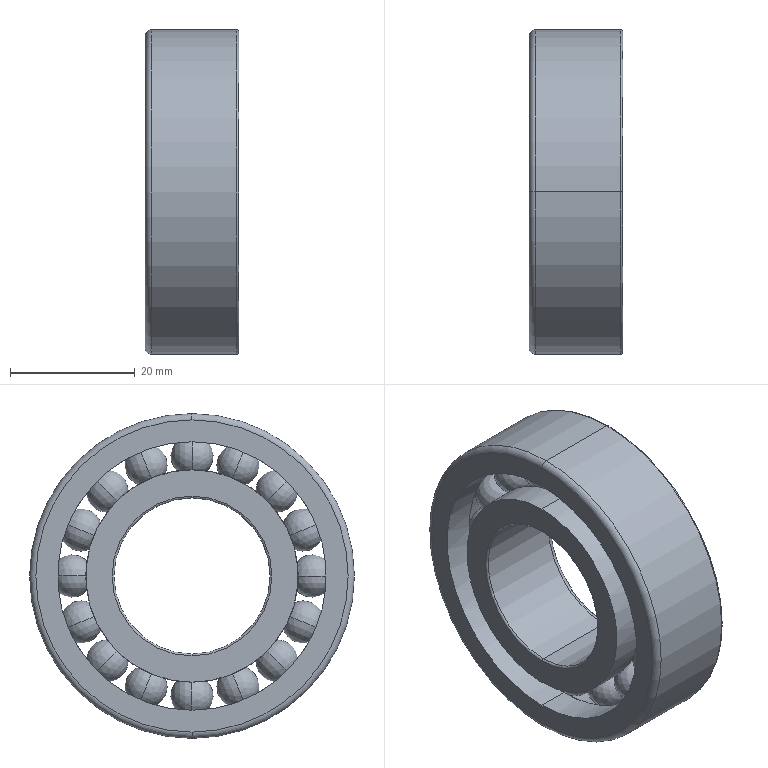Part | SolidWorks | features Stock 1 | 1 solid | 107 faces | box 15 x 52 x 52 mm | volume 17216 mm3 | torus 56 | sphere 32 | cylinder 14 | plane 5 | commonest cylinder face diameters 34 x4 25 x2 43 x2 44.29 x2 46.79 x2 52 x2